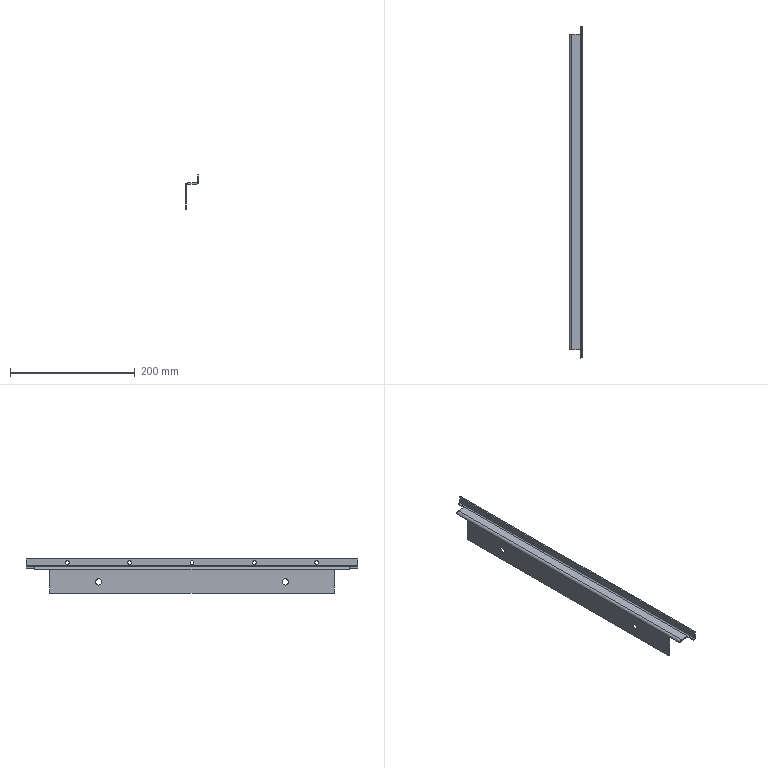Part | NX | features solid 2 | 1 solid | 36 faces | box 22 x 533 x 55 mm | volume 69859 mm3 | plane 18 | cylinder 18 | commonest cylinder face diameters 6 x10 10 x4 4 x2 8 x2
STEP:
#1=CARTESIAN_POINT('',(1088.,-73.,948.));
#2=VERTEX_POINT('',#1);
#3=CARTESIAN_POINT('',(1090.,-73.,950.));
#4=VERTEX_POINT('',#3);
#5=CARTESIAN_POINT('',(1090.,-73.,948.));
#6=DIRECTION('',(0.,1.,0.));
#7=DIRECTION('',(0.,0.,-1.));
#8=AXIS2_PLACEMENT_3D('',#5,#6,#7);
#9=CIRCLE('',#8,2.);
#10=EDGE_CURVE('',#2,#4,#9,.T.);
#11=ORIENTED_EDGE('',*,*,#10,.F.);
#12=CARTESIAN_POINT('',(1086.,-73.,948.));
#13=VERTEX_POINT('',#12);
#14=CARTESIAN_POINT('',(1088.,-73.,948.));
#15=DIRECTION('',(1.,0.,0.));
#16=VECTOR('',#15,1000.);
#17=LINE('',#14,#16);
#18=EDGE_CURVE('',#13,#2,#17,.T.);
#19=ORIENTED_EDGE('',*,*,#18,.F.);
#20=CARTESIAN_POINT('',(1090.,-73.,952.));
#21=VERTEX_POINT('',#20);
#22=CARTESIAN_POINT('',(1090.,-73.,948.));
#23=DIRECTION('',(0.,1.,0.));
#24=DIRECTION('',(0.,0.,-1.));
#25=AXIS2_PLACEMENT_3D('',#22,#23,#24);
#26=CIRCLE('',#25,4.);
#27=EDGE_CURVE('',#13,#21,#26,.T.);
#28=ORIENTED_EDGE('',*,*,#27,.T.);
#29=CARTESIAN_POINT('',(1104.,-73.,952.));
#30=VERTEX_POINT('',#29);
#31=CARTESIAN_POINT('',(1108.,-73.,952.));
#32=DIRECTION('',(1.,0.,0.));
#33=VECTOR('',#32,1000.);
#34=LINE('',#31,#33);
#35=EDGE_CURVE('',#21,#30,#34,.T.);
#36=ORIENTED_EDGE('',*,*,#35,.T.);
#37=CARTESIAN_POINT('',(1104.,-73.,950.));
#38=VERTEX_POINT('',#37);
#39=CARTESIAN_POINT('',(1104.,-73.,950.));
#40=DIRECTION('',(0.,0.,-1.));
#41=VECTOR('',#40,1000.);
#42=LINE('',#39,#41);
#43=EDGE_CURVE('',#30,#38,#42,.T.);
#44=ORIENTED_EDGE('',*,*,#43,.T.);
#45=CARTESIAN_POINT('',(1108.,-73.,950.));
#46=DIRECTION('',(1.,0.,0.));
#47=VECTOR('',#46,1000.);
#48=LINE('',#45,#47);
#49=EDGE_CURVE('',#4,#38,#48,.T.);
#50=ORIENTED_EDGE('',*,*,#49,.F.);
#51=EDGE_LOOP('',(#11,#19,#28,#36,#44,#50));
#52=FACE_BOUND('',#51,.T.);
#53=CARTESIAN_POINT('',(1090.,-73.,948.));
#54=DIRECTION('',(0.,1.,0.));
#55=DIRECTION('',(1.,0.,0.));
#56=AXIS2_PLACEMENT_3D('',#53,#54,#55);
#57=PLANE('',#56);
#58=ADVANCED_FACE('',(#52),#57,.T.);
#59=CARTESIAN_POINT('',(1104.,-60.,952.));
#60=VERTEX_POINT('',#59);
#61=CARTESIAN_POINT('',(1104.,-60.,950.));
#62=VERTEX_POINT('',#61);
#63=CARTESIAN_POINT('',(1104.,-60.,950.));
#64=DIRECTION('',(0.,0.,-1.));
#65=VECTOR('',#64,1000.);
#66=LINE('',#63,#65);
#67=EDGE_CURVE('',#60,#62,#66,.T.);
#68=ORIENTED_EDGE('',*,*,#67,.T.);
#69=CARTESIAN_POINT('',(1104.,-60.,950.));
#70=DIRECTION('',(0.,-1.,0.));
#71=VECTOR('',#70,1000.);
#72=LINE('',#69,#71);
#73=EDGE_CURVE('',#62,#38,#72,.T.);
#74=ORIENTED_EDGE('',*,*,#73,.T.);
#75=ORIENTED_EDGE('',*,*,#43,.F.);
#76=CARTESIAN_POINT('',(1104.,-60.,952.));
#77=DIRECTION('',(0.,-1.,0.));
#78=VECTOR('',#77,1000.);
#79=LINE('',#76,#78);
#80=EDGE_CURVE('',#60,#30,#79,.T.);
#81=ORIENTED_EDGE('',*,*,#80,.F.);
#82=EDGE_LOOP('',(#68,#74,#75,#81));
#83=FACE_BOUND('',#82,.T.);
#84=CARTESIAN_POINT('',(1104.,-60.,950.));
#85=DIRECTION('',(-1.,0.,0.));
#86=DIRECTION('',(0.,0.,1.));
#87=AXIS2_PLACEMENT_3D('',#84,#85,#86);
#88=PLANE('',#87);
#89=ADVANCED_FACE('',(#83),#88,.T.);
#90=CARTESIAN_POINT('',(1104.,-580.,952.));
#91=VERTEX_POINT('',#90);
#92=CARTESIAN_POINT('',(1090.,-580.,952.));
#93=VERTEX_POINT('',#92);
#94=CARTESIAN_POINT('',(1108.,-580.,952.));
#95=DIRECTION('',(-1.,0.,0.));
#96=VECTOR('',#95,1000.);
#97=LINE('',#94,#96);
#98=EDGE_CURVE('',#91,#93,#97,.T.);
#99=ORIENTED_EDGE('',*,*,#98,.T.);
#100=CARTESIAN_POINT('',(1086.,-580.,948.));
#101=VERTEX_POINT('',#100);
#102=CARTESIAN_POINT('',(1090.,-580.,948.));
#103=DIRECTION('',(0.,-1.,0.));
#104=DIRECTION('',(0.,0.,-1.));
#105=AXIS2_PLACEMENT_3D('',#102,#103,#104);
#106=CIRCLE('',#105,4.);
#107=EDGE_CURVE('',#93,#101,#106,.T.);
#108=ORIENTED_EDGE('',*,*,#107,.T.);
#109=CARTESIAN_POINT('',(1088.,-580.,948.));
#110=VERTEX_POINT('',#109);
#111=CARTESIAN_POINT('',(1088.,-580.,948.));
#112=DIRECTION('',(1.,0.,0.));
#113=VECTOR('',#112,1000.);
#114=LINE('',#111,#113);
#115=EDGE_CURVE('',#101,#110,#114,.T.);
#116=ORIENTED_EDGE('',*,*,#115,.T.);
#117=CARTESIAN_POINT('',(1090.,-580.,950.));
#118=VERTEX_POINT('',#117);
#119=CARTESIAN_POINT('',(1090.,-580.,948.));
#120=DIRECTION('',(0.,-1.,0.));
#121=DIRECTION('',(0.,0.,1.));
#122=AXIS2_PLACEMENT_3D('',#119,#120,#121);
#123=CIRCLE('',#122,2.);
#124=EDGE_CURVE('',#118,#110,#123,.T.);
#125=ORIENTED_EDGE('',*,*,#124,.F.);
#126=CARTESIAN_POINT('',(1104.,-580.,950.));
#127=VERTEX_POINT('',#126);
#128=CARTESIAN_POINT('',(1108.,-580.,950.));
#129=DIRECTION('',(-1.,0.,0.));
#130=VECTOR('',#129,1000.);
#131=LINE('',#128,#130);
#132=EDGE_CURVE('',#127,#118,#131,.T.);
#133=ORIENTED_EDGE('',*,*,#132,.F.);
#134=CARTESIAN_POINT('',(1104.,-580.,950.));
#135=DIRECTION('',(0.,0.,-1.));
#136=VECTOR('',#135,1000.);
#137=LINE('',#134,#136);
#138=EDGE_CURVE('',#91,#127,#137,.T.);
#139=ORIENTED_EDGE('',*,*,#138,.F.);
#140=EDGE_LOOP('',(#99,#108,#116,#125,#133,#139));
#141=FACE_BOUND('',#140,.T.);
#142=CARTESIAN_POINT('',(1108.,-580.,950.));
#143=DIRECTION('',(0.,1.,0.));
#144=DIRECTION('',(1.,0.,0.));
#145=AXIS2_PLACEMENT_3D('',#142,#143,#144);
#146=PLANE('',#145);
#147=ADVANCED_FACE('',(#141),#146,.F.);
#148=ORIENTED_EDGE('',*,*,#138,.T.);
#149=CARTESIAN_POINT('',(1104.,-593.,950.));
#150=VERTEX_POINT('',#149);
#151=CARTESIAN_POINT('',(1104.,-60.,950.));
#152=DIRECTION('',(0.,-1.,0.));
#153=VECTOR('',#152,1000.);
#154=LINE('',#151,#153);
#155=EDGE_CURVE('',#127,#150,#154,.T.);
#156=ORIENTED_EDGE('',*,*,#155,.T.);
#157=CARTESIAN_POINT('',(1104.,-593.,952.));
#158=VERTEX_POINT('',#157);
#159=CARTESIAN_POINT('',(1104.,-593.,950.));
#160=DIRECTION('',(0.,0.,-1.));
#161=VECTOR('',#160,1000.);
#162=LINE('',#159,#161);
#163=EDGE_CURVE('',#158,#150,#162,.T.);
#164=ORIENTED_EDGE('',*,*,#163,.F.);
#165=CARTESIAN_POINT('',(1104.,-60.,952.));
#166=DIRECTION('',(0.,-1.,0.));
#167=VECTOR('',#166,1000.);
#168=LINE('',#165,#167);
#169=EDGE_CURVE('',#91,#158,#168,.T.);
#170=ORIENTED_EDGE('',*,*,#169,.F.);
#171=EDGE_LOOP('',(#148,#156,#164,#170));
#172=FACE_BOUND('',#171,.T.);
#173=CARTESIAN_POINT('',(1104.,-60.,950.));
#174=DIRECTION('',(-1.,0.,0.));
#175=DIRECTION('',(0.,0.,1.));
#176=AXIS2_PLACEMENT_3D('',#173,#174,#175);
#177=PLANE('',#176);
#178=ADVANCED_FACE('',(#172),#177,.T.);
#179=CARTESIAN_POINT('',(1106.,-326.5,956.));
#180=VERTEX_POINT('',#179);
#181=CARTESIAN_POINT('',(1108.,-326.5,956.));
#182=VERTEX_POINT('',#181);
#183=CARTESIAN_POINT('',(1642.282,-326.5,956.));
#184=DIRECTION('',(-1.,0.,0.));
#185=VECTOR('',#184,1000.);
#186=LINE('',#183,#185);
#187=EDGE_CURVE('',#180,#182,#186,.F.);
#188=ORIENTED_EDGE('',*,*,#187,.T.);
#189=CARTESIAN_POINT('',(1108.,-326.5,962.));
#190=VERTEX_POINT('',#189);
#191=CARTESIAN_POINT('',(1108.,-326.5,959.));
#192=DIRECTION('',(-1.,0.,0.));
#193=DIRECTION('',(0.,0.,1.));
#194=AXIS2_PLACEMENT_3D('',#191,#192,#193);
#195=CIRCLE('',#194,3.);
#196=EDGE_CURVE('',#190,#182,#195,.T.);
#197=ORIENTED_EDGE('',*,*,#196,.F.);
#198=CARTESIAN_POINT('',(1106.,-326.5,962.));
#199=VERTEX_POINT('',#198);
#200=CARTESIAN_POINT('',(1642.282,-326.5,962.));
#201=DIRECTION('',(-1.,0.,0.));
#202=VECTOR('',#201,1000.);
#203=LINE('',#200,#202);
#204=EDGE_CURVE('',#190,#199,#203,.T.);
#205=ORIENTED_EDGE('',*,*,#204,.T.);
#206=CARTESIAN_POINT('',(1106.,-326.5,959.));
#207=DIRECTION('',(-1.,0.,0.));
#208=DIRECTION('',(0.,-1.,0.));
#209=AXIS2_PLACEMENT_3D('',#206,#207,#208);
#210=CIRCLE('',#209,3.);
#211=EDGE_CURVE('',#199,#180,#210,.T.);
#212=ORIENTED_EDGE('',*,*,#211,.T.);
#213=EDGE_LOOP('',(#188,#197,#205,#212));
#214=FACE_BOUND('',#213,.T.);
#215=CARTESIAN_POINT('',(1642.282,-326.5,959.));
#216=DIRECTION('',(-1.,0.,0.));
#217=DIRECTION('',(0.,0.,1.));
#218=AXIS2_PLACEMENT_3D('',#215,#216,#217);
#219=CYLINDRICAL_SURFACE('',#218,3.);
#220=ADVANCED_FACE('',(#214),#219,.F.);
#221=CARTESIAN_POINT('',(1106.,-126.5,956.));
#222=VERTEX_POINT('',#221);
#223=CARTESIAN_POINT('',(1108.,-126.5,956.));
#224=VERTEX_POINT('',#223);
#225=CARTESIAN_POINT('',(1642.282,-126.5,956.));
#226=DIRECTION('',(-1.,0.,0.));
#227=VECTOR('',#226,1000.);
#228=LINE('',#225,#227);
#229=EDGE_CURVE('',#222,#224,#228,.F.);
#230=ORIENTED_EDGE('',*,*,#229,.T.);
#231=CARTESIAN_POINT('',(1108.,-126.5,962.));
#232=VERTEX_POINT('',#231);
#233=CARTESIAN_POINT('',(1108.,-126.5,959.));
#234=DIRECTION('',(-1.,0.,0.));
#235=DIRECTION('',(0.,0.,1.));
#236=AXIS2_PLACEMENT_3D('',#233,#234,#235);
#237=CIRCLE('',#236,3.);
#238=EDGE_CURVE('',#232,#224,#237,.T.);
#239=ORIENTED_EDGE('',*,*,#238,.F.);
#240=CARTESIAN_POINT('',(1106.,-126.5,962.));
#241=VERTEX_POINT('',#240);
#242=CARTESIAN_POINT('',(1642.282,-126.5,962.));
#243=DIRECTION('',(-1.,0.,0.));
#244=VECTOR('',#243,1000.);
#245=LINE('',#242,#244);
#246=EDGE_CURVE('',#232,#241,#245,.T.);
#247=ORIENTED_EDGE('',*,*,#246,.T.);
#248=CARTESIAN_POINT('',(1106.,-126.5,959.));
#249=DIRECTION('',(-1.,0.,0.));
#250=DIRECTION('',(0.,-1.,0.));
#251=AXIS2_PLACEMENT_3D('',#248,#249,#250);
#252=CIRCLE('',#251,3.);
#253=EDGE_CURVE('',#241,#222,#252,.T.);
#254=ORIENTED_EDGE('',*,*,#253,.T.);
#255=EDGE_LOOP('',(#230,#239,#247,#254));
#256=FACE_BOUND('',#255,.T.);
#257=CARTESIAN_POINT('',(1642.282,-126.5,959.));
#258=DIRECTION('',(-1.,0.,0.));
#259=DIRECTION('',(0.,0.,1.));
#260=AXIS2_PLACEMENT_3D('',#257,#258,#259);
#261=CYLINDRICAL_SURFACE('',#260,3.);
#262=ADVANCED_FACE('',(#256),#261,.F.);
#263=CARTESIAN_POINT('',(1108.,-226.5,956.));
#264=VERTEX_POINT('',#263);
#265=CARTESIAN_POINT('',(1106.,-226.5,956.));
#266=VERTEX_POINT('',#265);
#267=CARTESIAN_POINT('',(1642.282,-226.5,956.));
#268=DIRECTION('',(-1.,0.,0.));
#269=VECTOR('',#268,1000.);
#270=LINE('',#267,#269);
#271=EDGE_CURVE('',#264,#266,#270,.T.);
#272=ORIENTED_EDGE('',*,*,#271,.F.);
#273=CARTESIAN_POINT('',(1108.,-226.5,962.));
#274=VERTEX_POINT('',#273);
#275=CARTESIAN_POINT('',(1108.,-226.5,959.));
#276=DIRECTION('',(-1.,0.,0.));
#277=DIRECTION('',(0.,0.,1.));
#278=AXIS2_PLACEMENT_3D('',#275,#276,#277);
#279=CIRCLE('',#278,3.);
#280=EDGE_CURVE('',#274,#264,#279,.T.);
#281=ORIENTED_EDGE('',*,*,#280,.F.);
#282=CARTESIAN_POINT('',(1106.,-226.5,962.));
#283=VERTEX_POINT('',#282);
#284=CARTESIAN_POINT('',(1642.282,-226.5,962.));
#285=DIRECTION('',(-1.,0.,0.));
#286=VECTOR('',#285,1000.);
#287=LINE('',#284,#286);
#288=EDGE_CURVE('',#283,#274,#287,.F.);
#289=ORIENTED_EDGE('',*,*,#288,.F.);
#290=CARTESIAN_POINT('',(1106.,-226.5,959.));
#291=DIRECTION('',(-1.,0.,0.));
#292=DIRECTION('',(0.,-1.,0.));
#293=AXIS2_PLACEMENT_3D('',#290,#291,#292);
#294=CIRCLE('',#293,3.);
#295=EDGE_CURVE('',#283,#266,#294,.T.);
#296=ORIENTED_EDGE('',*,*,#295,.T.);
#297=EDGE_LOOP('',(#272,#281,#289,#296));
#298=FACE_BOUND('',#297,.T.);
#299=CARTESIAN_POINT('',(1642.282,-226.5,959.));
#300=DIRECTION('',(-1.,0.,0.));
#301=DIRECTION('',(0.,0.,1.));
#302=AXIS2_PLACEMENT_3D('',#299,#300,#301);
#303=CYLINDRICAL_SURFACE('',#302,3.);
#304=ADVANCED_FACE('',(#298),#303,.F.);
#305=CARTESIAN_POINT('',(1106.,-526.5,956.));
#306=VERTEX_POINT('',#305);
#307=CARTESIAN_POINT('',(1108.,-526.5,956.));
#308=VERTEX_POINT('',#307);
#309=CARTESIAN_POINT('',(1642.282,-526.5,956.));
#310=DIRECTION('',(-1.,0.,0.));
#311=VECTOR('',#310,1000.);
#312=LINE('',#309,#311);
#313=EDGE_CURVE('',#306,#308,#312,.F.);
#314=ORIENTED_EDGE('',*,*,#313,.T.);
#315=CARTESIAN_POINT('',(1108.,-526.5,962.));
#316=VERTEX_POINT('',#315);
#317=CARTESIAN_POINT('',(1108.,-526.5,959.));
#318=DIRECTION('',(-1.,0.,0.));
#319=DIRECTION('',(0.,0.,1.));
#320=AXIS2_PLACEMENT_3D('',#317,#318,#319);
#321=CIRCLE('',#320,3.);
#322=EDGE_CURVE('',#316,#308,#321,.T.);
#323=ORIENTED_EDGE('',*,*,#322,.F.);
#324=CARTESIAN_POINT('',(1106.,-526.5,962.));
#325=VERTEX_POINT('',#324);
#326=CARTESIAN_POINT('',(1642.282,-526.5,962.));
#327=DIRECTION('',(-1.,0.,0.));
#328=VECTOR('',#327,1000.);
#329=LINE('',#326,#328);
#330=EDGE_CURVE('',#316,#325,#329,.T.);
#331=ORIENTED_EDGE('',*,*,#330,.T.);
#332=CARTESIAN_POINT('',(1106.,-526.5,959.));
#333=DIRECTION('',(-1.,0.,0.));
#334=DIRECTION('',(0.,-1.,0.));
#335=AXIS2_PLACEMENT_3D('',#332,#333,#334);
#336=CIRCLE('',#335,3.);
#337=EDGE_CURVE('',#325,#306,#336,.T.);
#338=ORIENTED_EDGE('',*,*,#337,.T.);
#339=EDGE_LOOP('',(#314,#323,#331,#338));
#340=FACE_BOUND('',#339,.T.);
#341=CARTESIAN_POINT('',(1642.282,-526.5,959.));
#342=DIRECTION('',(-1.,0.,0.));
#343=DIRECTION('',(0.,0.,1.));
#344=AXIS2_PLACEMENT_3D('',#341,#342,#343);
#345=CYLINDRICAL_SURFACE('',#344,3.);
#346=ADVANCED_FACE('',(#340),#345,.F.);
#347=CARTESIAN_POINT('',(1108.,-426.5,956.));
#348=VERTEX_POINT('',#347);
#349=CARTESIAN_POINT('',(1106.,-426.5,956.));
#350=VERTEX_POINT('',#349);
#351=CARTESIAN_POINT('',(1642.282,-426.5,956.));
#352=DIRECTION('',(-1.,0.,0.));
#353=VECTOR('',#352,1000.);
#354=LINE('',#351,#353);
#355=EDGE_CURVE('',#348,#350,#354,.T.);
#356=ORIENTED_EDGE('',*,*,#355,.F.);
#357=CARTESIAN_POINT('',(1108.,-426.5,962.));
#358=VERTEX_POINT('',#357);
#359=CARTESIAN_POINT('',(1108.,-426.5,959.));
#360=DIRECTION('',(-1.,0.,0.));
#361=DIRECTION('',(0.,0.,1.));
#362=AXIS2_PLACEMENT_3D('',#359,#360,#361);
#363=CIRCLE('',#362,3.);
#364=EDGE_CURVE('',#358,#348,#363,.T.);
#365=ORIENTED_EDGE('',*,*,#364,.F.);
#366=CARTESIAN_POINT('',(1106.,-426.5,962.));
#367=VERTEX_POINT('',#366);
#368=CARTESIAN_POINT('',(1642.282,-426.5,962.));
#369=DIRECTION('',(-1.,0.,0.));
#370=VECTOR('',#369,1000.);
#371=LINE('',#368,#370);
#372=EDGE_CURVE('',#367,#358,#371,.F.);
#373=ORIENTED_EDGE('',*,*,#372,.F.);
#374=CARTESIAN_POINT('',(1106.,-426.5,959.));
#375=DIRECTION('',(-1.,0.,0.));
#376=DIRECTION('',(0.,-1.,0.));
#377=AXIS2_PLACEMENT_3D('',#374,#375,#376);
#378=CIRCLE('',#377,3.);
#379=EDGE_CURVE('',#367,#350,#378,.T.);
#380=ORIENTED_EDGE('',*,*,#379,.T.);
#381=EDGE_LOOP('',(#356,#365,#373,#380));
#382=FACE_BOUND('',#381,.T.);
#383=CARTESIAN_POINT('',(1642.282,-426.5,959.));
#384=DIRECTION('',(-1.,0.,0.));
#385=DIRECTION('',(0.,0.,1.));
#386=AXIS2_PLACEMENT_3D('',#383,#384,#385);
#387=CYLINDRICAL_SURFACE('',#386,3.);
#388=ADVANCED_FACE('',(#382),#387,.F.);
#389=CARTESIAN_POINT('',(1086.,-476.5,933.));
#390=VERTEX_POINT('',#389);
#391=CARTESIAN_POINT('',(1088.,-476.5,933.));
#392=VERTEX_POINT('',#391);
#393=CARTESIAN_POINT('',(551.718,-476.5,933.));
#394=DIRECTION('',(1.,0.,0.));
#395=VECTOR('',#394,1000.);
#396=LINE('',#393,#395);
#397=EDGE_CURVE('',#390,#392,#396,.T.);
#398=ORIENTED_EDGE('',*,*,#397,.F.);
#399=CARTESIAN_POINT('',(1086.,-476.5,923.));
#400=VERTEX_POINT('',#399);
#401=CARTESIAN_POINT('',(1086.,-476.5,928.));
#402=DIRECTION('',(-1.,0.,0.));
#403=DIRECTION('',(0.,0.,1.));
#404=AXIS2_PLACEMENT_3D('',#401,#402,#403);
#405=CIRCLE('',#404,5.);
#406=EDGE_CURVE('',#390,#400,#405,.T.);
#407=ORIENTED_EDGE('',*,*,#406,.T.);
#408=CARTESIAN_POINT('',(1088.,-476.5,923.));
#409=VERTEX_POINT('',#408);
#410=CARTESIAN_POINT('',(551.718,-476.5,923.));
#411=DIRECTION('',(1.,0.,0.));
#412=VECTOR('',#411,1000.);
#413=LINE('',#410,#412);
#414=EDGE_CURVE('',#409,#400,#413,.F.);
#415=ORIENTED_EDGE('',*,*,#414,.F.);
#416=CARTESIAN_POINT('',(1088.,-476.5,928.));
#417=DIRECTION('',(1.,0.,0.));
#418=DIRECTION('',(0.,1.,0.));
#419=AXIS2_PLACEMENT_3D('',#416,#417,#418);
#420=CIRCLE('',#419,5.);
#421=EDGE_CURVE('',#409,#392,#420,.T.);
#422=ORIENTED_EDGE('',*,*,#421,.T.);
#423=EDGE_LOOP('',(#398,#407,#415,#422));
#424=FACE_BOUND('',#423,.T.);
#425=CARTESIAN_POINT('',(551.718,-476.5,928.));
#426=DIRECTION('',(1.,0.,0.));
#427=DIRECTION('',(0.,0.,-1.));
#428=AXIS2_PLACEMENT_3D('',#425,#426,#427);
#429=CYLINDRICAL_SURFACE('',#428,5.);
#430=ADVANCED_FACE('',(#424),#429,.F.);
#431=CARTESIAN_POINT('',(1088.,-176.5,933.));
#432=VERTEX_POINT('',#431);
#433=CARTESIAN_POINT('',(1086.,-176.5,933.));
#434=VERTEX_POINT('',#433);
#435=CARTESIAN_POINT('',(551.718,-176.5,933.));
#436=DIRECTION('',(1.,0.,0.));
#437=VECTOR('',#436,1000.);
#438=LINE('',#435,#437);
#439=EDGE_CURVE('',#432,#434,#438,.F.);
#440=ORIENTED_EDGE('',*,*,#439,.T.);
#441=CARTESIAN_POINT('',(1086.,-176.5,923.));
#442=VERTEX_POINT('',#441);
#443=CARTESIAN_POINT('',(1086.,-176.5,928.));
#444=DIRECTION('',(-1.,0.,0.));
#445=DIRECTION('',(0.,0.,1.));
#446=AXIS2_PLACEMENT_3D('',#443,#444,#445);
#447=CIRCLE('',#446,5.);
#448=EDGE_CURVE('',#434,#442,#447,.T.);
#449=ORIENTED_EDGE('',*,*,#448,.T.);
#450=CARTESIAN_POINT('',(1088.,-176.5,923.));
#451=VERTEX_POINT('',#450);
#452=CARTESIAN_POINT('',(551.718,-176.5,923.));
#453=DIRECTION('',(1.,0.,0.));
#454=VECTOR('',#453,1000.);
#455=LINE('',#452,#454);
#456=EDGE_CURVE('',#442,#451,#455,.T.);
#457=ORIENTED_EDGE('',*,*,#456,.T.);
#458=CARTESIAN_POINT('',(1088.,-176.5,928.));
#459=DIRECTION('',(1.,0.,0.));
#460=DIRECTION('',(0.,1.,0.));
#461=AXIS2_PLACEMENT_3D('',#458,#459,#460);
#462=CIRCLE('',#461,5.);
#463=EDGE_CURVE('',#451,#432,#462,.T.);
#464=ORIENTED_EDGE('',*,*,#463,.T.);
#465=EDGE_LOOP('',(#440,#449,#457,#464));
#466=FACE_BOUND('',#465,.T.);
#467=CARTESIAN_POINT('',(551.718,-176.5,928.));
#468=DIRECTION('',(1.,0.,0.));
#469=DIRECTION('',(0.,0.,-1.));
#470=AXIS2_PLACEMENT_3D('',#467,#468,#469);
#471=CYLINDRICAL_SURFACE('',#470,5.);
#472=ADVANCED_FACE('',(#466),#471,.F.);
#473=CARTESIAN_POINT('',(1086.,-98.,948.));
#474=VERTEX_POINT('',#473);
#475=CARTESIAN_POINT('',(1088.,-98.,948.));
#476=VERTEX_POINT('',#475);
#477=CARTESIAN_POINT('',(1088.,-98.,948.));
#478=DIRECTION('',(1.,0.,0.));
#479=VECTOR('',#478,1000.);
#480=LINE('',#477,#479);
#481=EDGE_CURVE('',#474,#476,#480,.T.);
#482=ORIENTED_EDGE('',*,*,#481,.T.);
#483=CARTESIAN_POINT('',(1088.,-98.,910.));
#484=VERTEX_POINT('',#483);
#485=CARTESIAN_POINT('',(1088.,-98.,950.));
#486=DIRECTION('',(0.,0.,1.));
#487=VECTOR('',#486,1000.);
#488=LINE('',#485,#487);
#489=EDGE_CURVE('',#484,#476,#488,.T.);
#490=ORIENTED_EDGE('',*,*,#489,.F.);
#491=CARTESIAN_POINT('',(1086.,-98.,910.));
#492=VERTEX_POINT('',#491);
#493=CARTESIAN_POINT('',(1088.,-98.,910.));
#494=DIRECTION('',(1.,0.,0.));
#495=VECTOR('',#494,1000.);
#496=LINE('',#493,#495);
#497=EDGE_CURVE('',#492,#484,#496,.T.);
#498=ORIENTED_EDGE('',*,*,#497,.F.);
#499=CARTESIAN_POINT('',(1086.,-98.,950.));
#500=DIRECTION('',(0.,0.,1.));
#501=VECTOR('',#500,1000.);
#502=LINE('',#499,#501);
#503=EDGE_CURVE('',#492,#474,#502,.T.);
#504=ORIENTED_EDGE('',*,*,#503,.T.);
#505=EDGE_LOOP('',(#482,#490,#498,#504));
#506=FACE_BOUND('',#505,.T.);
#507=CARTESIAN_POINT('',(1088.,-98.,950.));
#508=DIRECTION('',(0.,-1.,0.));
#509=DIRECTION('',(0.,0.,-1.));
#510=AXIS2_PLACEMENT_3D('',#507,#508,#509);
#511=PLANE('',#510);
#512=ADVANCED_FACE('',(#506),#511,.F.);
#513=CARTESIAN_POINT('',(1086.,-60.,948.));
#514=DIRECTION('',(0.,-1.,0.));
#515=VECTOR('',#514,1000.);
#516=LINE('',#513,#515);
#517=EDGE_CURVE('',#13,#474,#516,.T.);
#518=ORIENTED_EDGE('',*,*,#517,.F.);
#519=ORIENTED_EDGE('',*,*,#18,.T.);
#520=CARTESIAN_POINT('',(1088.,-60.,948.));
#521=DIRECTION('',(0.,-1.,0.));
#522=VECTOR('',#521,1000.);
#523=LINE('',#520,#522);
#524=EDGE_CURVE('',#2,#476,#523,.T.);
#525=ORIENTED_EDGE('',*,*,#524,.T.);
#526=ORIENTED_EDGE('',*,*,#481,.F.);
#527=EDGE_LOOP('',(#518,#519,#525,#526));
#528=FACE_BOUND('',#527,.T.);
#529=CARTESIAN_POINT('',(1088.,-60.,948.));
#530=DIRECTION('',(0.,0.,-1.));
#531=DIRECTION('',(0.,-1.,0.));
#532=AXIS2_PLACEMENT_3D('',#529,#530,#531);
#533=PLANE('',#532);
#534=ADVANCED_FACE('',(#528),#533,.T.);
#535=CARTESIAN_POINT('',(1086.,-555.,910.));
#536=VERTEX_POINT('',#535);
#537=CARTESIAN_POINT('',(1086.,-555.,948.));
#538=VERTEX_POINT('',#537);
#539=CARTESIAN_POINT('',(1086.,-555.,950.));
#540=DIRECTION('',(0.,0.,1.));
#541=VECTOR('',#540,1000.);
#542=LINE('',#539,#541);
#543=EDGE_CURVE('',#536,#538,#542,.T.);
#544=ORIENTED_EDGE('',*,*,#543,.F.);
#545=CARTESIAN_POINT('',(1088.,-555.,910.));
#546=VERTEX_POINT('',#545);
#547=CARTESIAN_POINT('',(1088.,-555.,910.));
#548=DIRECTION('',(1.,0.,0.));
#549=VECTOR('',#548,1000.);
#550=LINE('',#547,#549);
#551=EDGE_CURVE('',#536,#546,#550,.T.);
#552=ORIENTED_EDGE('',*,*,#551,.T.);
#553=CARTESIAN_POINT('',(1088.,-555.,948.));
#554=VERTEX_POINT('',#553);
#555=CARTESIAN_POINT('',(1088.,-555.,950.));
#556=DIRECTION('',(0.,0.,1.));
#557=VECTOR('',#556,1000.);
#558=LINE('',#555,#557);
#559=EDGE_CURVE('',#546,#554,#558,.T.);
#560=ORIENTED_EDGE('',*,*,#559,.T.);
#561=CARTESIAN_POINT('',(1088.,-555.,948.));
#562=DIRECTION('',(1.,0.,0.));
#563=VECTOR('',#562,1000.);
#564=LINE('',#561,#563);
#565=EDGE_CURVE('',#538,#554,#564,.T.);
#566=ORIENTED_EDGE('',*,*,#565,.F.);
#567=EDGE_LOOP('',(#544,#552,#560,#566));
#568=FACE_BOUND('',#567,.T.);
#569=CARTESIAN_POINT('',(1088.,-555.,950.));
#570=DIRECTION('',(0.,-1.,0.));
#571=DIRECTION('',(0.,0.,-1.));
#572=AXIS2_PLACEMENT_3D('',#569,#570,#571);
#573=PLANE('',#572);
#574=ADVANCED_FACE('',(#568),#573,.T.);
#575=ORIENTED_EDGE('',*,*,#463,.F.);
#576=CARTESIAN_POINT('',(1088.,-176.5,928.));
#577=DIRECTION('',(1.,0.,0.));
#578=DIRECTION('',(0.,1.,0.));
#579=AXIS2_PLACEMENT_3D('',#576,#577,#578);
#580=CIRCLE('',#579,5.);
#581=EDGE_CURVE('',#432,#451,#580,.T.);
#582=ORIENTED_EDGE('',*,*,#581,.F.);
#583=EDGE_LOOP('',(#575,#582));
#584=FACE_BOUND('',#583,.T.);
#585=ORIENTED_EDGE('',*,*,#421,.F.);
#586=CARTESIAN_POINT('',(1088.,-476.5,928.));
#587=DIRECTION('',(1.,0.,0.));
#588=DIRECTION('',(0.,1.,0.));
#589=AXIS2_PLACEMENT_3D('',#586,#587,#588);
#590=CIRCLE('',#589,5.);
#591=EDGE_CURVE('',#392,#409,#590,.T.);
#592=ORIENTED_EDGE('',*,*,#591,.F.);
#593=EDGE_LOOP('',(#585,#592));
#594=FACE_BOUND('',#593,.T.);
#595=CARTESIAN_POINT('',(1088.,-60.,910.));
#596=DIRECTION('',(0.,-1.,0.));
#597=VECTOR('',#596,1000.);
#598=LINE('',#595,#597);
#599=EDGE_CURVE('',#484,#546,#598,.T.);
#600=ORIENTED_EDGE('',*,*,#599,.F.);
#601=ORIENTED_EDGE('',*,*,#489,.T.);
#602=CARTESIAN_POINT('',(1088.,-60.,948.));
#603=DIRECTION('',(0.,-1.,0.));
#604=VECTOR('',#603,1000.);
#605=LINE('',#602,#604);
#606=EDGE_CURVE('',#476,#554,#605,.T.);
#607=ORIENTED_EDGE('',*,*,#606,.T.);
#608=ORIENTED_EDGE('',*,*,#559,.F.);
#609=EDGE_LOOP('',(#600,#601,#607,#608));
#610=FACE_BOUND('',#609,.T.);
#611=CARTESIAN_POINT('',(1088.,-60.,950.));
#612=DIRECTION('',(-1.,0.,0.));
#613=DIRECTION('',(0.,0.,1.));
#614=AXIS2_PLACEMENT_3D('',#611,#612,#613);
#615=PLANE('',#614);
#616=ADVANCED_FACE('',(#584,#594,#610),#615,.F.);
#617=ORIENTED_EDGE('',*,*,#524,.F.);
#618=ORIENTED_EDGE('',*,*,#10,.T.);
#619=CARTESIAN_POINT('',(1090.,-60.,950.));
#620=DIRECTION('',(0.,-1.,0.));
#621=VECTOR('',#620,1000.);
#622=LINE('',#619,#621);
#623=EDGE_CURVE('',#4,#118,#622,.T.);
#624=ORIENTED_EDGE('',*,*,#623,.T.);
#625=ORIENTED_EDGE('',*,*,#124,.T.);
#626=CARTESIAN_POINT('',(1088.,-60.,948.));
#627=DIRECTION('',(0.,-1.,0.));
#628=VECTOR('',#627,1000.);
#629=LINE('',#626,#628);
#630=EDGE_CURVE('',#554,#110,#629,.T.);
#631=ORIENTED_EDGE('',*,*,#630,.F.);
#632=ORIENTED_EDGE('',*,*,#606,.F.);
#633=EDGE_LOOP('',(#617,#618,#624,#625,#631,#632));
#634=FACE_BOUND('',#633,.T.);
#635=CARTESIAN_POINT('',(1090.,-60.,948.));
#636=DIRECTION('',(0.,-1.,0.));
#637=DIRECTION('',(0.,0.,-1.));
#638=AXIS2_PLACEMENT_3D('',#635,#636,#637);
#639=CYLINDRICAL_SURFACE('',#638,2.);
#640=ADVANCED_FACE('',(#634),#639,.F.);
#641=ORIENTED_EDGE('',*,*,#623,.F.);
#642=ORIENTED_EDGE('',*,*,#49,.T.);
#643=CARTESIAN_POINT('',(1104.,-60.,950.));
#644=DIRECTION('',(0.,-1.,0.));
#645=VECTOR('',#644,1000.);
#646=LINE('',#643,#645);
#647=EDGE_CURVE('',#38,#127,#646,.T.);
#648=ORIENTED_EDGE('',*,*,#647,.T.);
#649=ORIENTED_EDGE('',*,*,#132,.T.);
#650=EDGE_LOOP('',(#641,#642,#648,#649));
#651=FACE_BOUND('',#650,.T.);
#652=CARTESIAN_POINT('',(1108.,-60.,950.));
#653=DIRECTION('',(0.,0.,1.));
#654=DIRECTION('',(1.,0.,0.));
#655=AXIS2_PLACEMENT_3D('',#652,#653,#654);
#656=PLANE('',#655);
#657=ADVANCED_FACE('',(#651),#656,.F.);
#658=CARTESIAN_POINT('',(1108.,-593.,954.));
#659=VERTEX_POINT('',#658);
#660=CARTESIAN_POINT('',(1104.,-593.,954.));
#661=DIRECTION('',(0.,1.,0.));
#662=DIRECTION('',(0.,0.,-1.));
#663=AXIS2_PLACEMENT_3D('',#660,#661,#662);
#664=CIRCLE('',#663,4.);
#665=EDGE_CURVE('',#659,#150,#664,.T.);
#666=ORIENTED_EDGE('',*,*,#665,.T.);
#667=ORIENTED_EDGE('',*,*,#155,.F.);
#668=ORIENTED_EDGE('',*,*,#647,.F.);
#669=ORIENTED_EDGE('',*,*,#73,.F.);
#670=CARTESIAN_POINT('',(1108.,-60.,954.));
#671=VERTEX_POINT('',#670);
#672=CARTESIAN_POINT('',(1104.,-60.,954.));
#673=DIRECTION('',(0.,1.,0.));
#674=DIRECTION('',(0.,0.,-1.));
#675=AXIS2_PLACEMENT_3D('',#672,#673,#674);
#676=CIRCLE('',#675,4.);
#677=EDGE_CURVE('',#671,#62,#676,.T.);
#678=ORIENTED_EDGE('',*,*,#677,.F.);
#679=CARTESIAN_POINT('',(1108.,-60.,954.));
#680=DIRECTION('',(0.,-1.,0.));
#681=VECTOR('',#680,1000.);
#682=LINE('',#679,#681);
#683=EDGE_CURVE('',#671,#659,#682,.T.);
#684=ORIENTED_EDGE('',*,*,#683,.T.);
#685=EDGE_LOOP('',(#666,#667,#668,#669,#678,#684));
#686=FACE_BOUND('',#685,.T.);
#687=CARTESIAN_POINT('',(1104.,-60.,954.));
#688=DIRECTION('',(0.,-1.,0.));
#689=DIRECTION('',(0.,0.,-1.));
#690=AXIS2_PLACEMENT_3D('',#687,#688,#689);
#691=CYLINDRICAL_SURFACE('',#690,4.);
#692=ADVANCED_FACE('',(#686),#691,.T.);
#693=ORIENTED_EDGE('',*,*,#364,.T.);
#694=CARTESIAN_POINT('',(1108.,-426.5,959.));
#695=DIRECTION('',(-1.,0.,0.));
#696=DIRECTION('',(0.,0.,1.));
#697=AXIS2_PLACEMENT_3D('',#694,#695,#696);
#698=CIRCLE('',#697,3.);
#699=EDGE_CURVE('',#348,#358,#698,.T.);
#700=ORIENTED_EDGE('',*,*,#699,.T.);
#701=EDGE_LOOP('',(#693,#700));
#702=FACE_BOUND('',#701,.T.);
#703=ORIENTED_EDGE('',*,*,#322,.T.);
#704=CARTESIAN_POINT('',(1108.,-526.5,959.));
#705=DIRECTION('',(-1.,0.,0.));
#706=DIRECTION('',(0.,0.,1.));
#707=AXIS2_PLACEMENT_3D('',#704,#705,#706);
#708=CIRCLE('',#707,3.);
#709=EDGE_CURVE('',#308,#316,#708,.T.);
#710=ORIENTED_EDGE('',*,*,#709,.T.);
#711=EDGE_LOOP('',(#703,#710));
#712=FACE_BOUND('',#711,.T.);
#713=ORIENTED_EDGE('',*,*,#280,.T.);
#714=CARTESIAN_POINT('',(1108.,-226.5,959.));
#715=DIRECTION('',(-1.,0.,0.));
#716=DIRECTION('',(0.,0.,1.));
#717=AXIS2_PLACEMENT_3D('',#714,#715,#716);
#718=CIRCLE('',#717,3.);
#719=EDGE_CURVE('',#264,#274,#718,.T.);
#720=ORIENTED_EDGE('',*,*,#719,.T.);
#721=EDGE_LOOP('',(#713,#720));
#722=FACE_BOUND('',#721,.T.);
#723=ORIENTED_EDGE('',*,*,#238,.T.);
#724=CARTESIAN_POINT('',(1108.,-126.5,959.));
#725=DIRECTION('',(-1.,0.,0.));
#726=DIRECTION('',(0.,0.,1.));
#727=AXIS2_PLACEMENT_3D('',#724,#725,#726);
#728=CIRCLE('',#727,3.);
#729=EDGE_CURVE('',#224,#232,#728,.T.);
#730=ORIENTED_EDGE('',*,*,#729,.T.);
#731=EDGE_LOOP('',(#723,#730));
#732=FACE_BOUND('',#731,.T.);
#733=ORIENTED_EDGE('',*,*,#196,.T.);
#734=CARTESIAN_POINT('',(1108.,-326.5,959.));
#735=DIRECTION('',(-1.,0.,0.));
#736=DIRECTION('',(0.,0.,1.));
#737=AXIS2_PLACEMENT_3D('',#734,#735,#736);
#738=CIRCLE('',#737,3.);
#739=EDGE_CURVE('',#182,#190,#738,.T.);
#740=ORIENTED_EDGE('',*,*,#739,.T.);
#741=EDGE_LOOP('',(#733,#740));
#742=FACE_BOUND('',#741,.T.);
#743=CARTESIAN_POINT('',(1108.,-593.,965.));
#744=VERTEX_POINT('',#743);
#745=CARTESIAN_POINT('',(1108.,-593.,965.));
#746=DIRECTION('',(0.,0.,-1.));
#747=VECTOR('',#746,1000.);
#748=LINE('',#745,#747);
#749=EDGE_CURVE('',#744,#659,#748,.T.);
#750=ORIENTED_EDGE('',*,*,#749,.T.);
#751=ORIENTED_EDGE('',*,*,#683,.F.);
#752=CARTESIAN_POINT('',(1108.,-60.,965.));
#753=VERTEX_POINT('',#752);
#754=CARTESIAN_POINT('',(1108.,-60.,965.));
#755=DIRECTION('',(0.,0.,-1.));
#756=VECTOR('',#755,1000.);
#757=LINE('',#754,#756);
#758=EDGE_CURVE('',#753,#671,#757,.T.);
#759=ORIENTED_EDGE('',*,*,#758,.F.);
#760=CARTESIAN_POINT('',(1108.,-60.,965.));
#761=DIRECTION('',(0.,-1.,0.));
#762=VECTOR('',#761,1000.);
#763=LINE('',#760,#762);
#764=EDGE_CURVE('',#753,#744,#763,.T.);
#765=ORIENTED_EDGE('',*,*,#764,.T.);
#766=EDGE_LOOP('',(#750,#751,#759,#765));
#767=FACE_BOUND('',#766,.T.);
#768=CARTESIAN_POINT('',(1108.,-60.,965.));
#769=DIRECTION('',(-1.,0.,0.));
#770=DIRECTION('',(0.,0.,1.));
#771=AXIS2_PLACEMENT_3D('',#768,#769,#770);
#772=PLANE('',#771);
#773=ADVANCED_FACE('',(#702,#712,#722,#732,#742,#767),#772,.F.);
#774=CARTESIAN_POINT('',(1086.,-176.5,928.));
#775=DIRECTION('',(-1.,0.,0.));
#776=DIRECTION('',(0.,0.,1.));
#777=AXIS2_PLACEMENT_3D('',#774,#775,#776);
#778=CIRCLE('',#777,5.);
#779=EDGE_CURVE('',#442,#434,#778,.T.);
#780=ORIENTED_EDGE('',*,*,#779,.F.);
#781=ORIENTED_EDGE('',*,*,#448,.F.);
#782=EDGE_LOOP('',(#780,#781));
#783=FACE_BOUND('',#782,.T.);
#784=CARTESIAN_POINT('',(1086.,-476.5,928.));
#785=DIRECTION('',(-1.,0.,0.));
#786=DIRECTION('',(0.,0.,1.));
#787=AXIS2_PLACEMENT_3D('',#784,#785,#786);
#788=CIRCLE('',#787,5.);
#789=EDGE_CURVE('',#400,#390,#788,.T.);
#790=ORIENTED_EDGE('',*,*,#789,.F.);
#791=ORIENTED_EDGE('',*,*,#406,.F.);
#792=EDGE_LOOP('',(#790,#791));
#793=FACE_BOUND('',#792,.T.);
#794=ORIENTED_EDGE('',*,*,#503,.F.);
#795=CARTESIAN_POINT('',(1086.,-60.,910.));
#796=DIRECTION('',(0.,-1.,0.));
#797=VECTOR('',#796,1000.);
#798=LINE('',#795,#797);
#799=EDGE_CURVE('',#492,#536,#798,.T.);
#800=ORIENTED_EDGE('',*,*,#799,.T.);
#801=ORIENTED_EDGE('',*,*,#543,.T.);
#802=CARTESIAN_POINT('',(1086.,-60.,948.));
#803=DIRECTION('',(0.,-1.,0.));
#804=VECTOR('',#803,1000.);
#805=LINE('',#802,#804);
#806=EDGE_CURVE('',#474,#538,#805,.T.);
#807=ORIENTED_EDGE('',*,*,#806,.F.);
#808=EDGE_LOOP('',(#794,#800,#801,#807));
#809=FACE_BOUND('',#808,.T.);
#810=CARTESIAN_POINT('',(1086.,-60.,950.));
#811=DIRECTION('',(-1.,0.,0.));
#812=DIRECTION('',(0.,0.,1.));
#813=AXIS2_PLACEMENT_3D('',#810,#811,#812);
#814=PLANE('',#813);
#815=ADVANCED_FACE('',(#783,#793,#809),#814,.T.);
#816=ORIENTED_EDGE('',*,*,#27,.F.);
#817=ORIENTED_EDGE('',*,*,#517,.T.);
#818=ORIENTED_EDGE('',*,*,#806,.T.);
#819=CARTESIAN_POINT('',(1086.,-60.,948.));
#820=DIRECTION('',(0.,-1.,0.));
#821=VECTOR('',#820,1000.);
#822=LINE('',#819,#821);
#823=EDGE_CURVE('',#538,#101,#822,.T.);
#824=ORIENTED_EDGE('',*,*,#823,.T.);
#825=ORIENTED_EDGE('',*,*,#107,.F.);
#826=CARTESIAN_POINT('',(1090.,-60.,952.));
#827=DIRECTION('',(0.,-1.,0.));
#828=VECTOR('',#827,1000.);
#829=LINE('',#826,#828);
#830=EDGE_CURVE('',#21,#93,#829,.T.);
#831=ORIENTED_EDGE('',*,*,#830,.F.);
#832=EDGE_LOOP('',(#816,#817,#818,#824,#825,#831));
#833=FACE_BOUND('',#832,.T.);
#834=CARTESIAN_POINT('',(1090.,-60.,948.));
#835=DIRECTION('',(0.,-1.,0.));
#836=DIRECTION('',(0.,0.,-1.));
#837=AXIS2_PLACEMENT_3D('',#834,#835,#836);
#838=CYLINDRICAL_SURFACE('',#837,4.);
#839=ADVANCED_FACE('',(#833),#838,.T.);
#840=ORIENTED_EDGE('',*,*,#35,.F.);
#841=ORIENTED_EDGE('',*,*,#830,.T.);
#842=ORIENTED_EDGE('',*,*,#98,.F.);
#843=CARTESIAN_POINT('',(1104.,-60.,952.));
#844=DIRECTION('',(0.,-1.,0.));
#845=VECTOR('',#844,1000.);
#846=LINE('',#843,#845);
#847=EDGE_CURVE('',#30,#91,#846,.T.);
#848=ORIENTED_EDGE('',*,*,#847,.F.);
#849=EDGE_LOOP('',(#840,#841,#842,#848));
#850=FACE_BOUND('',#849,.T.);
#851=CARTESIAN_POINT('',(1108.,-60.,952.));
#852=DIRECTION('',(0.,0.,1.));
#853=DIRECTION('',(1.,0.,0.));
#854=AXIS2_PLACEMENT_3D('',#851,#852,#853);
#855=PLANE('',#854);
#856=ADVANCED_FACE('',(#850),#855,.T.);
#857=CARTESIAN_POINT('',(1106.,-593.,954.));
#858=VERTEX_POINT('',#857);
#859=CARTESIAN_POINT('',(1104.,-593.,954.));
#860=DIRECTION('',(0.,1.,0.));
#861=DIRECTION('',(0.,0.,-1.));
#862=AXIS2_PLACEMENT_3D('',#859,#860,#861);
#863=CIRCLE('',#862,2.);
#864=EDGE_CURVE('',#858,#158,#863,.T.);
#865=ORIENTED_EDGE('',*,*,#864,.F.);
#866=CARTESIAN_POINT('',(1106.,-60.,954.));
#867=VERTEX_POINT('',#866);
#868=CARTESIAN_POINT('',(1106.,-60.,954.));
#869=DIRECTION('',(0.,-1.,0.));
#870=VECTOR('',#869,1000.);
#871=LINE('',#868,#870);
#872=EDGE_CURVE('',#867,#858,#871,.T.);
#873=ORIENTED_EDGE('',*,*,#872,.F.);
#874=CARTESIAN_POINT('',(1104.,-60.,954.));
#875=DIRECTION('',(0.,1.,0.));
#876=DIRECTION('',(0.,0.,-1.));
#877=AXIS2_PLACEMENT_3D('',#874,#875,#876);
#878=CIRCLE('',#877,2.);
#879=EDGE_CURVE('',#867,#60,#878,.T.);
#880=ORIENTED_EDGE('',*,*,#879,.T.);
#881=ORIENTED_EDGE('',*,*,#80,.T.);
#882=ORIENTED_EDGE('',*,*,#847,.T.);
#883=ORIENTED_EDGE('',*,*,#169,.T.);
#884=EDGE_LOOP('',(#865,#873,#880,#881,#882,#883));
#885=FACE_BOUND('',#884,.T.);
#886=CARTESIAN_POINT('',(1104.,-60.,954.));
#887=DIRECTION('',(0.,-1.,0.));
#888=DIRECTION('',(0.,0.,-1.));
#889=AXIS2_PLACEMENT_3D('',#886,#887,#888);
#890=CYLINDRICAL_SURFACE('',#889,2.);
#891=ADVANCED_FACE('',(#885),#890,.F.);
#892=ORIENTED_EDGE('',*,*,#379,.F.);
#893=CARTESIAN_POINT('',(1106.,-426.5,959.));
#894=DIRECTION('',(-1.,0.,0.));
#895=DIRECTION('',(0.,-1.,0.));
#896=AXIS2_PLACEMENT_3D('',#893,#894,#895);
#897=CIRCLE('',#896,3.);
#898=EDGE_CURVE('',#350,#367,#897,.T.);
#899=ORIENTED_EDGE('',*,*,#898,.F.);
#900=EDGE_LOOP('',(#892,#899));
#901=FACE_BOUND('',#900,.T.);
#902=ORIENTED_EDGE('',*,*,#337,.F.);
#903=CARTESIAN_POINT('',(1106.,-526.5,959.));
#904=DIRECTION('',(-1.,0.,0.));
#905=DIRECTION('',(0.,-1.,0.));
#906=AXIS2_PLACEMENT_3D('',#903,#904,#905);
#907=CIRCLE('',#906,3.);
#908=EDGE_CURVE('',#306,#325,#907,.T.);
#909=ORIENTED_EDGE('',*,*,#908,.F.);
#910=EDGE_LOOP('',(#902,#909));
#911=FACE_BOUND('',#910,.T.);
#912=ORIENTED_EDGE('',*,*,#295,.F.);
#913=CARTESIAN_POINT('',(1106.,-226.5,959.));
#914=DIRECTION('',(-1.,0.,0.));
#915=DIRECTION('',(0.,-1.,0.));
#916=AXIS2_PLACEMENT_3D('',#913,#914,#915);
#917=CIRCLE('',#916,3.);
#918=EDGE_CURVE('',#266,#283,#917,.T.);
#919=ORIENTED_EDGE('',*,*,#918,.F.);
#920=EDGE_LOOP('',(#912,#919));
#921=FACE_BOUND('',#920,.T.);
#922=ORIENTED_EDGE('',*,*,#253,.F.);
#923=CARTESIAN_POINT('',(1106.,-126.5,959.));
#924=DIRECTION('',(-1.,0.,0.));
#925=DIRECTION('',(0.,-1.,0.));
#926=AXIS2_PLACEMENT_3D('',#923,#924,#925);
#927=CIRCLE('',#926,3.);
#928=EDGE_CURVE('',#222,#241,#927,.T.);
#929=ORIENTED_EDGE('',*,*,#928,.F.);
#930=EDGE_LOOP('',(#922,#929));
#931=FACE_BOUND('',#930,.T.);
#932=ORIENTED_EDGE('',*,*,#211,.F.);
#933=CARTESIAN_POINT('',(1106.,-326.5,959.));
#934=DIRECTION('',(-1.,0.,0.));
#935=DIRECTION('',(0.,-1.,0.));
#936=AXIS2_PLACEMENT_3D('',#933,#934,#935);
#937=CIRCLE('',#936,3.);
#938=EDGE_CURVE('',#180,#199,#937,.T.);
#939=ORIENTED_EDGE('',*,*,#938,.F.);
#940=EDGE_LOOP('',(#932,#939));
#941=FACE_BOUND('',#940,.T.);
#942=CARTESIAN_POINT('',(1106.,-593.,965.));
#943=VERTEX_POINT('',#942);
#944=CARTESIAN_POINT('',(1106.,-593.,965.));
#945=DIRECTION('',(0.,0.,-1.));
#946=VECTOR('',#945,1000.);
#947=LINE('',#944,#946);
#948=EDGE_CURVE('',#943,#858,#947,.T.);
#949=ORIENTED_EDGE('',*,*,#948,.F.);
#950=CARTESIAN_POINT('',(1106.,-60.,965.));
#951=VERTEX_POINT('',#950);
#952=CARTESIAN_POINT('',(1106.,-60.,965.));
#953=DIRECTION('',(0.,-1.,0.));
#954=VECTOR('',#953,1000.);
#955=LINE('',#952,#954);
#956=EDGE_CURVE('',#951,#943,#955,.T.);
#957=ORIENTED_EDGE('',*,*,#956,.F.);
#958=CARTESIAN_POINT('',(1106.,-60.,965.));
#959=DIRECTION('',(0.,0.,-1.));
#960=VECTOR('',#959,1000.);
#961=LINE('',#958,#960);
#962=EDGE_CURVE('',#951,#867,#961,.T.);
#963=ORIENTED_EDGE('',*,*,#962,.T.);
#964=ORIENTED_EDGE('',*,*,#872,.T.);
#965=EDGE_LOOP('',(#949,#957,#963,#964));
#966=FACE_BOUND('',#965,.T.);
#967=CARTESIAN_POINT('',(1106.,-60.,965.));
#968=DIRECTION('',(-1.,0.,0.));
#969=DIRECTION('',(0.,0.,1.));
#970=AXIS2_PLACEMENT_3D('',#967,#968,#969);
#971=PLANE('',#970);
#972=ADVANCED_FACE('',(#901,#911,#921,#931,#941,#966),#971,.T.);
#973=ORIENTED_EDGE('',*,*,#764,.F.);
#974=CARTESIAN_POINT('',(1108.,-60.,965.));
#975=DIRECTION('',(-1.,0.,0.));
#976=VECTOR('',#975,1000.);
#977=LINE('',#974,#976);
#978=EDGE_CURVE('',#753,#951,#977,.T.);
#979=ORIENTED_EDGE('',*,*,#978,.T.);
#980=ORIENTED_EDGE('',*,*,#956,.T.);
#981=CARTESIAN_POINT('',(1108.,-593.,965.));
#982=DIRECTION('',(-1.,0.,0.));
#983=VECTOR('',#982,1000.);
#984=LINE('',#981,#983);
#985=EDGE_CURVE('',#744,#943,#984,.T.);
#986=ORIENTED_EDGE('',*,*,#985,.F.);
#987=EDGE_LOOP('',(#973,#979,#980,#986));
#988=FACE_BOUND('',#987,.T.);
#989=CARTESIAN_POINT('',(1108.,-60.,965.));
#990=DIRECTION('',(0.,0.,-1.));
#991=DIRECTION('',(0.,-1.,0.));
#992=AXIS2_PLACEMENT_3D('',#989,#990,#991);
#993=PLANE('',#992);
#994=ADVANCED_FACE('',(#988),#993,.F.);
#995=ORIENTED_EDGE('',*,*,#67,.F.);
#996=ORIENTED_EDGE('',*,*,#879,.F.);
#997=ORIENTED_EDGE('',*,*,#962,.F.);
#998=ORIENTED_EDGE('',*,*,#978,.F.);
#999=ORIENTED_EDGE('',*,*,#758,.T.);
#1000=ORIENTED_EDGE('',*,*,#677,.T.);
#1001=EDGE_LOOP('',(#995,#996,#997,#998,#999,#1000));
#1002=FACE_BOUND('',#1001,.T.);
#1003=CARTESIAN_POINT('',(1088.,-60.,950.));
#1004=DIRECTION('',(0.,1.,0.));
#1005=DIRECTION('',(1.,0.,0.));
#1006=AXIS2_PLACEMENT_3D('',#1003,#1004,#1005);
#1007=PLANE('',#1006);
#1008=ADVANCED_FACE('',(#1002),#1007,.T.);
#1009=ORIENTED_EDGE('',*,*,#799,.F.);
#1010=ORIENTED_EDGE('',*,*,#497,.T.);
#1011=ORIENTED_EDGE('',*,*,#599,.T.);
#1012=ORIENTED_EDGE('',*,*,#551,.F.);
#1013=EDGE_LOOP('',(#1009,#1010,#1011,#1012));
#1014=FACE_BOUND('',#1013,.T.);
#1015=CARTESIAN_POINT('',(1088.,-60.,910.));
#1016=DIRECTION('',(0.,0.,-1.));
#1017=DIRECTION('',(0.,-1.,0.));
#1018=AXIS2_PLACEMENT_3D('',#1015,#1016,#1017);
#1019=PLANE('',#1018);
#1020=ADVANCED_FACE('',(#1014),#1019,.T.);
#1021=ORIENTED_EDGE('',*,*,#115,.F.);
#1022=ORIENTED_EDGE('',*,*,#823,.F.);
#1023=ORIENTED_EDGE('',*,*,#565,.T.);
#1024=ORIENTED_EDGE('',*,*,#630,.T.);
#1025=EDGE_LOOP('',(#1021,#1022,#1023,#1024));
#1026=FACE_BOUND('',#1025,.T.);
#1027=CARTESIAN_POINT('',(1088.,-60.,948.));
#1028=DIRECTION('',(0.,0.,-1.));
#1029=DIRECTION('',(0.,-1.,0.));
#1030=AXIS2_PLACEMENT_3D('',#1027,#1028,#1029);
#1031=PLANE('',#1030);
#1032=ADVANCED_FACE('',(#1026),#1031,.T.);
#1033=ORIENTED_EDGE('',*,*,#864,.T.);
#1034=ORIENTED_EDGE('',*,*,#163,.T.);
#1035=ORIENTED_EDGE('',*,*,#665,.F.);
#1036=ORIENTED_EDGE('',*,*,#749,.F.);
#1037=ORIENTED_EDGE('',*,*,#985,.T.);
#1038=ORIENTED_EDGE('',*,*,#948,.T.);
#1039=EDGE_LOOP('',(#1033,#1034,#1035,#1036,#1037,#1038));
#1040=FACE_BOUND('',#1039,.T.);
#1041=CARTESIAN_POINT('',(1108.,-593.,965.));
#1042=DIRECTION('',(0.,1.,0.));
#1043=DIRECTION('',(1.,0.,0.));
#1044=AXIS2_PLACEMENT_3D('',#1041,#1042,#1043);
#1045=PLANE('',#1044);
#1046=ADVANCED_FACE('',(#1040),#1045,.F.);
#1047=ORIENTED_EDGE('',*,*,#779,.T.);
#1048=ORIENTED_EDGE('',*,*,#439,.F.);
#1049=ORIENTED_EDGE('',*,*,#581,.T.);
#1050=ORIENTED_EDGE('',*,*,#456,.F.);
#1051=EDGE_LOOP('',(#1047,#1048,#1049,#1050));
#1052=FACE_BOUND('',#1051,.T.);
#1053=CARTESIAN_POINT('',(551.718,-176.5,928.));
#1054=DIRECTION('',(1.,0.,0.));
#1055=DIRECTION('',(0.,0.,-1.));
#1056=AXIS2_PLACEMENT_3D('',#1053,#1054,#1055);
#1057=CYLINDRICAL_SURFACE('',#1056,5.);
#1058=ADVANCED_FACE('',(#1052),#1057,.F.);
#1059=ORIENTED_EDGE('',*,*,#789,.T.);
#1060=ORIENTED_EDGE('',*,*,#397,.T.);
#1061=ORIENTED_EDGE('',*,*,#591,.T.);
#1062=ORIENTED_EDGE('',*,*,#414,.T.);
#1063=EDGE_LOOP('',(#1059,#1060,#1061,#1062));
#1064=FACE_BOUND('',#1063,.T.);
#1065=CARTESIAN_POINT('',(551.718,-476.5,928.));
#1066=DIRECTION('',(1.,0.,0.));
#1067=DIRECTION('',(0.,0.,-1.));
#1068=AXIS2_PLACEMENT_3D('',#1065,#1066,#1067);
#1069=CYLINDRICAL_SURFACE('',#1068,5.);
#1070=ADVANCED_FACE('',(#1064),#1069,.F.);
#1071=ORIENTED_EDGE('',*,*,#699,.F.);
#1072=ORIENTED_EDGE('',*,*,#355,.T.);
#1073=ORIENTED_EDGE('',*,*,#898,.T.);
#1074=ORIENTED_EDGE('',*,*,#372,.T.);
#1075=EDGE_LOOP('',(#1071,#1072,#1073,#1074));
#1076=FACE_BOUND('',#1075,.T.);
#1077=CARTESIAN_POINT('',(1642.282,-426.5,959.));
#1078=DIRECTION('',(-1.,0.,0.));
#1079=DIRECTION('',(0.,0.,1.));
#1080=AXIS2_PLACEMENT_3D('',#1077,#1078,#1079);
#1081=CYLINDRICAL_SURFACE('',#1080,3.);
#1082=ADVANCED_FACE('',(#1076),#1081,.F.);
#1083=ORIENTED_EDGE('',*,*,#709,.F.);
#1084=ORIENTED_EDGE('',*,*,#313,.F.);
#1085=ORIENTED_EDGE('',*,*,#908,.T.);
#1086=ORIENTED_EDGE('',*,*,#330,.F.);
#1087=EDGE_LOOP('',(#1083,#1084,#1085,#1086));
#1088=FACE_BOUND('',#1087,.T.);
#1089=CARTESIAN_POINT('',(1642.282,-526.5,959.));
#1090=DIRECTION('',(-1.,0.,0.));
#1091=DIRECTION('',(0.,0.,1.));
#1092=AXIS2_PLACEMENT_3D('',#1089,#1090,#1091);
#1093=CYLINDRICAL_SURFACE('',#1092,3.);
#1094=ADVANCED_FACE('',(#1088),#1093,.F.);
#1095=ORIENTED_EDGE('',*,*,#719,.F.);
#1096=ORIENTED_EDGE('',*,*,#271,.T.);
#1097=ORIENTED_EDGE('',*,*,#918,.T.);
#1098=ORIENTED_EDGE('',*,*,#288,.T.);
#1099=EDGE_LOOP('',(#1095,#1096,#1097,#1098));
#1100=FACE_BOUND('',#1099,.T.);
#1101=CARTESIAN_POINT('',(1642.282,-226.5,959.));
#1102=DIRECTION('',(-1.,0.,0.));
#1103=DIRECTION('',(0.,0.,1.));
#1104=AXIS2_PLACEMENT_3D('',#1101,#1102,#1103);
#1105=CYLINDRICAL_SURFACE('',#1104,3.);
#1106=ADVANCED_FACE('',(#1100),#1105,.F.);
#1107=ORIENTED_EDGE('',*,*,#729,.F.);
#1108=ORIENTED_EDGE('',*,*,#229,.F.);
#1109=ORIENTED_EDGE('',*,*,#928,.T.);
#1110=ORIENTED_EDGE('',*,*,#246,.F.);
#1111=EDGE_LOOP('',(#1107,#1108,#1109,#1110));
#1112=FACE_BOUND('',#1111,.T.);
#1113=CARTESIAN_POINT('',(1642.282,-126.5,959.));
#1114=DIRECTION('',(-1.,0.,0.));
#1115=DIRECTION('',(0.,0.,1.));
#1116=AXIS2_PLACEMENT_3D('',#1113,#1114,#1115);
#1117=CYLINDRICAL_SURFACE('',#1116,3.);
#1118=ADVANCED_FACE('',(#1112),#1117,.F.);
#1119=ORIENTED_EDGE('',*,*,#739,.F.);
#1120=ORIENTED_EDGE('',*,*,#187,.F.);
#1121=ORIENTED_EDGE('',*,*,#938,.T.);
#1122=ORIENTED_EDGE('',*,*,#204,.F.);
#1123=EDGE_LOOP('',(#1119,#1120,#1121,#1122));
#1124=FACE_BOUND('',#1123,.T.);
#1125=CARTESIAN_POINT('',(1642.282,-326.5,959.));
#1126=DIRECTION('',(-1.,0.,0.));
#1127=DIRECTION('',(0.,0.,1.));
#1128=AXIS2_PLACEMENT_3D('',#1125,#1126,#1127);
#1129=CYLINDRICAL_SURFACE('',#1128,3.);
#1130=ADVANCED_FACE('',(#1124),#1129,.F.);
#1131=CLOSED_SHELL('',(#58,#89,#147,#178,#220,#262,#304,#346,#388,#430,#472,#512,#534,#574,#616,#640,#657,#692,#773,#815,#839,#856,#891,#972,#994,#1008,#1020,#1032,#1046,#1058,#1070,#1082,#1094,#1106,#1118,#1130));
#1132=MANIFOLD_SOLID_BREP('',#1131);
#1133=(LENGTH_UNIT()NAMED_UNIT(*)SI_UNIT(.MILLI.,.METRE.));
#1134=UNCERTAINTY_MEASURE_WITH_UNIT(LENGTH_MEASURE(0.00001),#1133,'','');
#1135=(NAMED_UNIT(*)PLANE_ANGLE_UNIT()SI_UNIT($,.RADIAN.));
#1136=(NAMED_UNIT(*)SI_UNIT($,.STERADIAN.)SOLID_ANGLE_UNIT());
#1137=(GEOMETRIC_REPRESENTATION_CONTEXT(3)GLOBAL_UNCERTAINTY_ASSIGNED_CONTEXT((#1134))GLOBAL_UNIT_ASSIGNED_CONTEXT((#1133,#1135,#1136))REPRESENTATION_CONTEXT('',''));
#1138=ADVANCED_BREP_SHAPE_REPRESENTATION('',(#1132),#1137);